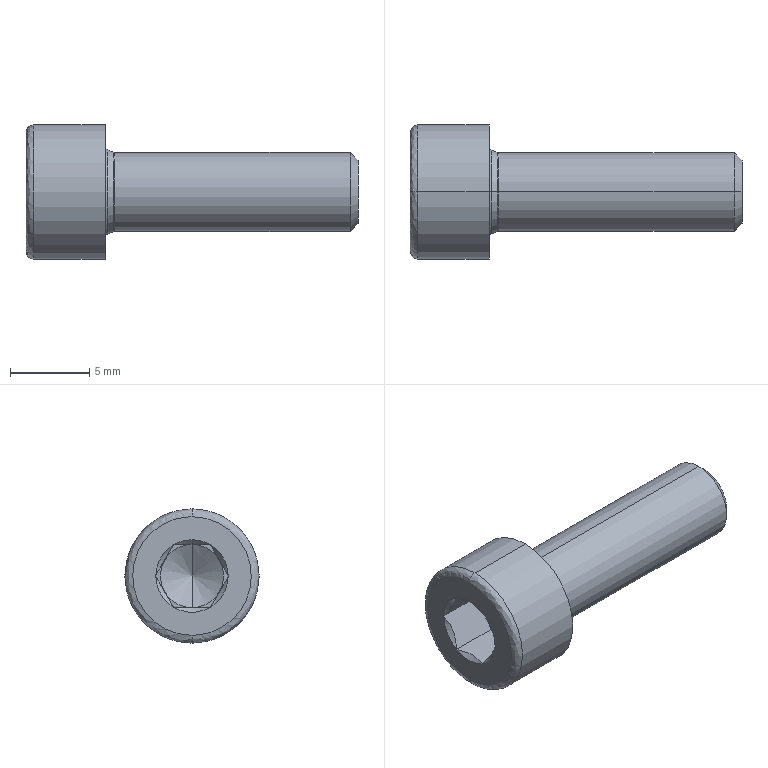Part | STEP file | _Hexagon socket head cap screw DIN 912 - M5x16 | 1 solid | 38 faces | box 21 x 8.5 x 8.5 mm | volume 547.668 mm3 | plane 15 | cone 13 | spline 6 | cylinder 4 | commonest cylinder face diameters 5 x2 8.5 x2
STEP:
#1=CARTESIAN_POINT('',(0.5298,0.,2.513));
#2=VERTEX_POINT('',#1);
#3=CARTESIAN_POINT('',(0.5298,0.,-2.513));
#4=VERTEX_POINT('',#3);
#5=CARTESIAN_POINT('',(0.5298,0.,0.));
#6=DIRECTION('',(-1.,0.,0.));
#7=DIRECTION('',(0.,0.,-1.));
#8=AXIS2_PLACEMENT_3D('',#5,#6,#7);
#9=CIRCLE('',#8,2.513);
#10=EDGE_CURVE('',#2,#4,#9,.T.);
#11=ORIENTED_EDGE('',*,*,#10,.F.);
#12=CARTESIAN_POINT('',(0.6,0.,2.5));
#13=VERTEX_POINT('',#12);
#14=CARTESIAN_POINT('',(0.6,0.,2.7));
#15=DIRECTION('',(0.,-1.,0.));
#16=DIRECTION('',(0.,0.,1.));
#17=AXIS2_PLACEMENT_3D('',#14,#15,#16);
#18=CIRCLE('',#17,0.2);
#19=EDGE_CURVE('',#2,#13,#18,.T.);
#20=ORIENTED_EDGE('',*,*,#19,.T.);
#21=CARTESIAN_POINT('',(0.6,0.,-2.5));
#22=VERTEX_POINT('',#21);
#23=CARTESIAN_POINT('',(0.6,0.,0.));
#24=DIRECTION('',(1.,0.,0.));
#25=DIRECTION('',(0.,0.,1.));
#26=AXIS2_PLACEMENT_3D('',#23,#24,#25);
#27=CIRCLE('',#26,2.5);
#28=EDGE_CURVE('',#22,#13,#27,.T.);
#29=ORIENTED_EDGE('',*,*,#28,.F.);
#30=CARTESIAN_POINT('',(0.6,0.,-2.7));
#31=DIRECTION('',(0.,1.,0.));
#32=DIRECTION('',(0.,0.,-1.));
#33=AXIS2_PLACEMENT_3D('',#30,#31,#32);
#34=CIRCLE('',#33,0.2);
#35=EDGE_CURVE('',#4,#22,#34,.T.);
#36=ORIENTED_EDGE('',*,*,#35,.F.);
#37=EDGE_LOOP('',(#11,#20,#29,#36));
#38=FACE_OUTER_BOUND('',#37,.T.);
#39=CARTESIAN_POINT('',(0.5298,0.,-2.513));
#40=CARTESIAN_POINT('',(0.5298,5.025,-2.513));
#41=CARTESIAN_POINT('',(0.5298,5.025,2.513));
#42=CARTESIAN_POINT('',(0.5298,0.,2.513));
#43=CARTESIAN_POINT('',(0.5523,0.,-2.504));
#44=CARTESIAN_POINT('',(0.5523,5.009,-2.504));
#45=CARTESIAN_POINT('',(0.5523,5.009,2.504));
#46=CARTESIAN_POINT('',(0.5523,0.,2.504));
#47=CARTESIAN_POINT('',(0.576,0.,-2.5));
#48=CARTESIAN_POINT('',(0.576,5.,-2.5));
#49=CARTESIAN_POINT('',(0.576,5.,2.5));
#50=CARTESIAN_POINT('',(0.576,0.,2.5));
#51=CARTESIAN_POINT('',(0.6,0.,-2.5));
#52=CARTESIAN_POINT('',(0.6,5.,-2.5));
#53=CARTESIAN_POINT('',(0.6,5.,2.5));
#54=CARTESIAN_POINT('',(0.6,0.,2.5));
#55=(BOUNDED_SURFACE()B_SPLINE_SURFACE(3,3,((#39,#40,#41,#42),(#43,#44,#45,#46),(#47,#48,#49,#50),(#51,#52,#53,#54)),.UNSPECIFIED.,.F.,.F.,.F.)B_SPLINE_SURFACE_WITH_KNOTS((4,4),(4,4),(0.,1.),(0.,1.),.UNSPECIFIED.)GEOMETRIC_REPRESENTATION_ITEM()RATIONAL_B_SPLINE_SURFACE(((1.,0.3333,0.3333,1.),(0.9893,0.3298,0.3298,0.9893),(0.9893,0.3298,0.3298,0.9893),(1.,0.3333,0.3333,1.)))REPRESENTATION_ITEM('')SURFACE());
#56=ADVANCED_FACE('',(#38),#55,.F.);
#57=CARTESIAN_POINT('',(0.,0.,2.85));
#58=VERTEX_POINT('',#57);
#59=CARTESIAN_POINT('',(0.,0.,-2.85));
#60=VERTEX_POINT('',#59);
#61=CARTESIAN_POINT('',(0.,0.,2.85));
#62=CARTESIAN_POINT('',(0.,0.1814,2.85));
#63=CARTESIAN_POINT('',(0.,0.4486,2.825));
#64=CARTESIAN_POINT('',(0.,0.7517,2.752));
#65=CARTESIAN_POINT('',(0.,0.9011,2.705));
#66=CARTESIAN_POINT('',(0.,0.9647,2.682));
#67=CARTESIAN_POINT('',(0.,1.007,2.666));
#68=CARTESIAN_POINT('',(0.,1.026,2.659));
#69=CARTESIAN_POINT('',(0.,1.415,2.505));
#70=CARTESIAN_POINT('',(0.,1.737,2.294));
#71=CARTESIAN_POINT('',(0.,2.154,1.876));
#72=CARTESIAN_POINT('',(0.,2.338,1.651));
#73=CARTESIAN_POINT('',(0.,2.509,1.359));
#74=CARTESIAN_POINT('',(0.,2.583,1.207));
#75=CARTESIAN_POINT('',(0.,2.612,1.14));
#76=CARTESIAN_POINT('',(0.,2.632,1.095));
#77=CARTESIAN_POINT('',(0.,2.642,1.07));
#78=CARTESIAN_POINT('',(0.,2.783,0.7118));
#79=CARTESIAN_POINT('',(0.,2.85,0.3628));
#80=CARTESIAN_POINT('',(0.,2.85,-0.1814));
#81=CARTESIAN_POINT('',(0.,2.825,-0.4486));
#82=CARTESIAN_POINT('',(0.,2.752,-0.7517));
#83=CARTESIAN_POINT('',(0.,2.705,-0.9011));
#84=CARTESIAN_POINT('',(0.,2.682,-0.9647));
#85=CARTESIAN_POINT('',(0.,2.666,-1.007));
#86=CARTESIAN_POINT('',(0.,2.659,-1.026));
#87=CARTESIAN_POINT('',(0.,2.505,-1.415));
#88=CARTESIAN_POINT('',(0.,2.294,-1.737));
#89=CARTESIAN_POINT('',(0.,1.876,-2.154));
#90=CARTESIAN_POINT('',(0.,1.651,-2.338));
#91=CARTESIAN_POINT('',(0.,1.359,-2.509));
#92=CARTESIAN_POINT('',(0.,1.207,-2.583));
#93=CARTESIAN_POINT('',(0.,1.14,-2.612));
#94=CARTESIAN_POINT('',(0.,1.095,-2.632));
#95=CARTESIAN_POINT('',(0.,1.07,-2.642));
#96=CARTESIAN_POINT('',(0.,0.7119,-2.783));
#97=CARTESIAN_POINT('',(0.,0.3622,-2.85));
#98=CARTESIAN_POINT('',(0.,0.,-2.85));
#99=B_SPLINE_CURVE_WITH_KNOTS('',3,(#61,#62,#63,#64,#65,#66,#67,#68,#69,#70,#71,#72,#73,#74,#75,#76,#77,#78,#79,#80,#81,#82,#83,#84,#85,#86,#87,#88,#89,#90,#91,#92,#93,#94,#95,#96,#97,#98),.UNSPECIFIED.,.F.,.F.,(4,1,1,1,2,2,2,1,1,1,2,2,2,1,1,1,2,2,2,1,1,1,2,2,4),(0.5,0.5312,0.5469,0.5547,0.5586,0.5625,0.625,0.6562,0.6719,0.6797,0.6836,0.6875,0.75,0.7812,0.7969,0.8047,0.8086,0.8125,0.875,0.9062,0.9219,0.9297,0.9336,0.9375,1.),.UNSPECIFIED.);
#100=EDGE_CURVE('',#58,#60,#99,.T.);
#101=ORIENTED_EDGE('',*,*,#100,.F.);
#102=CARTESIAN_POINT('',(0.1298,0.,2.663));
#103=VERTEX_POINT('',#102);
#104=CARTESIAN_POINT('',(0.2,0.,2.85));
#105=DIRECTION('',(0.,-1.,0.));
#106=DIRECTION('',(0.,0.,1.));
#107=AXIS2_PLACEMENT_3D('',#104,#105,#106);
#108=CIRCLE('',#107,0.2);
#109=EDGE_CURVE('',#58,#103,#108,.T.);
#110=ORIENTED_EDGE('',*,*,#109,.T.);
#111=CARTESIAN_POINT('',(0.1298,0.,-2.663));
#112=VERTEX_POINT('',#111);
#113=CARTESIAN_POINT('',(0.1298,0.,0.));
#114=DIRECTION('',(1.,0.,0.));
#115=DIRECTION('',(0.,0.,1.));
#116=AXIS2_PLACEMENT_3D('',#113,#114,#115);
#117=CIRCLE('',#116,2.663);
#118=EDGE_CURVE('',#112,#103,#117,.T.);
#119=ORIENTED_EDGE('',*,*,#118,.F.);
#120=CARTESIAN_POINT('',(0.2,0.,-2.85));
#121=DIRECTION('',(0.,1.,0.));
#122=DIRECTION('',(0.,0.,-1.));
#123=AXIS2_PLACEMENT_3D('',#120,#121,#122);
#124=CIRCLE('',#123,0.2);
#125=EDGE_CURVE('',#60,#112,#124,.T.);
#126=ORIENTED_EDGE('',*,*,#125,.F.);
#127=EDGE_LOOP('',(#101,#110,#119,#126));
#128=FACE_OUTER_BOUND('',#127,.T.);
#129=CARTESIAN_POINT('',(0.,0.,-2.85));
#130=CARTESIAN_POINT('',(0.,5.7,-2.85));
#131=CARTESIAN_POINT('',(0.,5.7,2.85));
#132=CARTESIAN_POINT('',(0.,0.,2.85));
#133=CARTESIAN_POINT('',(0.,0.,-2.764));
#134=CARTESIAN_POINT('',(0.,5.528,-2.764));
#135=CARTESIAN_POINT('',(0.,5.528,2.764));
#136=CARTESIAN_POINT('',(0.,0.,2.764));
#137=CARTESIAN_POINT('',(0.04909,0.,-2.693));
#138=CARTESIAN_POINT('',(0.04909,5.386,-2.693));
#139=CARTESIAN_POINT('',(0.04909,5.386,2.693));
#140=CARTESIAN_POINT('',(0.04909,0.,2.693));
#141=CARTESIAN_POINT('',(0.1298,0.,-2.663));
#142=CARTESIAN_POINT('',(0.1298,5.325,-2.663));
#143=CARTESIAN_POINT('',(0.1298,5.325,2.663));
#144=CARTESIAN_POINT('',(0.1298,0.,2.663));
#145=(BOUNDED_SURFACE()B_SPLINE_SURFACE(3,3,((#129,#130,#131,#132),(#133,#134,#135,#136),(#137,#138,#139,#140),(#141,#142,#143,#144)),.UNSPECIFIED.,.F.,.F.,.T.)B_SPLINE_SURFACE_WITH_KNOTS((4,4),(4,4),(0.,1.),(0.,1.),.UNSPECIFIED.)GEOMETRIC_REPRESENTATION_ITEM()RATIONAL_B_SPLINE_SURFACE(((1.,0.3333,0.3333,1.),(0.8813,0.2938,0.2938,0.8813),(0.8813,0.2938,0.2938,0.8813),(1.,0.3333,0.3333,1.)))REPRESENTATION_ITEM('')SURFACE());
#146=ADVANCED_FACE('',(#128),#145,.F.);
#147=CARTESIAN_POINT('',(-4.5,0.,4.25));
#148=VERTEX_POINT('',#147);
#149=CARTESIAN_POINT('',(-4.5,0.,-4.25));
#150=VERTEX_POINT('',#149);
#151=CARTESIAN_POINT('',(-4.5,0.,0.));
#152=DIRECTION('',(1.,0.,0.));
#153=DIRECTION('',(0.,0.,1.));
#154=AXIS2_PLACEMENT_3D('',#151,#152,#153);
#155=CIRCLE('',#154,4.25);
#156=EDGE_CURVE('',#148,#150,#155,.T.);
#157=ORIENTED_EDGE('',*,*,#156,.F.);
#158=CARTESIAN_POINT('',(-5.,0.,3.75));
#159=VERTEX_POINT('',#158);
#160=CARTESIAN_POINT('',(-4.5,0.,3.75));
#161=DIRECTION('',(0.,-1.,0.));
#162=DIRECTION('',(0.,0.,1.));
#163=AXIS2_PLACEMENT_3D('',#160,#161,#162);
#164=CIRCLE('',#163,0.5);
#165=EDGE_CURVE('',#148,#159,#164,.T.);
#166=ORIENTED_EDGE('',*,*,#165,.T.);
#167=CARTESIAN_POINT('',(-5.,0.,-3.75));
#168=VERTEX_POINT('',#167);
#169=CARTESIAN_POINT('',(-5.,0.,3.75));
#170=CARTESIAN_POINT('',(-5.,-7.5,3.75));
#171=CARTESIAN_POINT('',(-5.,-7.5,-3.75));
#172=CARTESIAN_POINT('',(-5.,0.,-3.75));
#173=(BOUNDED_CURVE()B_SPLINE_CURVE(3,(#169,#170,#171,#172),.UNSPECIFIED.,.F.,.F.)B_SPLINE_CURVE_WITH_KNOTS((4,4),(0.5,1.),.UNSPECIFIED.)CURVE()GEOMETRIC_REPRESENTATION_ITEM()RATIONAL_B_SPLINE_CURVE((1.,0.3333,0.3333,1.))REPRESENTATION_ITEM(''));
#174=EDGE_CURVE('',#159,#168,#173,.T.);
#175=ORIENTED_EDGE('',*,*,#174,.T.);
#176=CARTESIAN_POINT('',(-4.5,0.,-3.75));
#177=DIRECTION('',(0.,1.,0.));
#178=DIRECTION('',(0.,0.,-1.));
#179=AXIS2_PLACEMENT_3D('',#176,#177,#178);
#180=CIRCLE('',#179,0.5);
#181=EDGE_CURVE('',#150,#168,#180,.T.);
#182=ORIENTED_EDGE('',*,*,#181,.F.);
#183=EDGE_LOOP('',(#157,#166,#175,#182));
#184=FACE_OUTER_BOUND('',#183,.T.);
#185=CARTESIAN_POINT('',(-4.5,0.,4.25));
#186=CARTESIAN_POINT('',(-4.5,-8.5,4.25));
#187=CARTESIAN_POINT('',(-4.5,-8.5,-4.25));
#188=CARTESIAN_POINT('',(-4.5,0.,-4.25));
#189=CARTESIAN_POINT('',(-4.793,0.,4.25));
#190=CARTESIAN_POINT('',(-4.793,-8.5,4.25));
#191=CARTESIAN_POINT('',(-4.793,-8.5,-4.25));
#192=CARTESIAN_POINT('',(-4.793,0.,-4.25));
#193=CARTESIAN_POINT('',(-5.,0.,4.043));
#194=CARTESIAN_POINT('',(-5.,-8.086,4.043));
#195=CARTESIAN_POINT('',(-5.,-8.086,-4.043));
#196=CARTESIAN_POINT('',(-5.,0.,-4.043));
#197=CARTESIAN_POINT('',(-5.,0.,3.75));
#198=CARTESIAN_POINT('',(-5.,-7.5,3.75));
#199=CARTESIAN_POINT('',(-5.,-7.5,-3.75));
#200=CARTESIAN_POINT('',(-5.,0.,-3.75));
#201=(BOUNDED_SURFACE()B_SPLINE_SURFACE(3,3,((#185,#186,#187,#188),(#189,#190,#191,#192),(#193,#194,#195,#196),(#197,#198,#199,#200)),.UNSPECIFIED.,.F.,.F.,.F.)B_SPLINE_SURFACE_WITH_KNOTS((4,4),(4,4),(0.,1.),(0.,1.),.UNSPECIFIED.)GEOMETRIC_REPRESENTATION_ITEM()RATIONAL_B_SPLINE_SURFACE(((1.,0.3333,0.3333,1.),(0.8047,0.2682,0.2682,0.8047),(0.8047,0.2682,0.2682,0.8047),(1.,0.3333,0.3333,1.)))REPRESENTATION_ITEM('')SURFACE());
#202=ADVANCED_FACE('',(#184),#201,.T.);
#203=CARTESIAN_POINT('',(15.509,0.,2.5));
#204=VERTEX_POINT('',#203);
#205=CARTESIAN_POINT('',(15.509,0.,-2.5));
#206=VERTEX_POINT('',#205);
#207=CARTESIAN_POINT('',(15.509,0.,0.));
#208=DIRECTION('',(-1.,0.,0.));
#209=DIRECTION('',(0.,0.,1.));
#210=AXIS2_PLACEMENT_3D('',#207,#208,#209);
#211=CIRCLE('',#210,2.5);
#212=EDGE_CURVE('',#204,#206,#211,.T.);
#213=ORIENTED_EDGE('',*,*,#212,.T.);
#214=CARTESIAN_POINT('',(19.,0.,-2.5));
#215=DIRECTION('',(-1.,0.,0.));
#216=VECTOR('',#215,1000.);
#217=LINE('',#214,#216);
#218=EDGE_CURVE('',#206,#22,#217,.T.);
#219=ORIENTED_EDGE('',*,*,#218,.T.);
#220=ORIENTED_EDGE('',*,*,#28,.T.);
#221=CARTESIAN_POINT('',(19.,0.,2.5));
#222=DIRECTION('',(-1.,0.,0.));
#223=VECTOR('',#222,1000.);
#224=LINE('',#221,#223);
#225=EDGE_CURVE('',#204,#13,#224,.T.);
#226=ORIENTED_EDGE('',*,*,#225,.F.);
#227=EDGE_LOOP('',(#213,#219,#220,#226));
#228=FACE_OUTER_BOUND('',#227,.T.);
#229=CARTESIAN_POINT('',(19.,0.,0.));
#230=DIRECTION('',(-1.,0.,0.));
#231=DIRECTION('',(0.,0.,1.));
#232=AXIS2_PLACEMENT_3D('',#229,#230,#231);
#233=CYLINDRICAL_SURFACE('',#232,2.5);
#234=ADVANCED_FACE('',(#228),#233,.T.);
#235=CARTESIAN_POINT('',(16.,0.,2.009));
#236=VERTEX_POINT('',#235);
#237=CARTESIAN_POINT('',(16.,0.,-2.009));
#238=VERTEX_POINT('',#237);
#239=CARTESIAN_POINT('',(16.,0.,0.));
#240=DIRECTION('',(-1.,0.,0.));
#241=DIRECTION('',(0.,0.,1.));
#242=AXIS2_PLACEMENT_3D('',#239,#240,#241);
#243=CIRCLE('',#242,2.009);
#244=EDGE_CURVE('',#236,#238,#243,.T.);
#245=ORIENTED_EDGE('',*,*,#244,.T.);
#246=CARTESIAN_POINT('',(15.51,0.,-2.5));
#247=DIRECTION('',(-0.7071,0.,-0.7071));
#248=VECTOR('',#247,1000.);
#249=LINE('',#246,#248);
#250=EDGE_CURVE('',#238,#206,#249,.T.);
#251=ORIENTED_EDGE('',*,*,#250,.T.);
#252=ORIENTED_EDGE('',*,*,#212,.F.);
#253=CARTESIAN_POINT('',(15.51,0.,2.5));
#254=DIRECTION('',(-0.7071,0.,0.7071));
#255=VECTOR('',#254,1000.);
#256=LINE('',#253,#255);
#257=EDGE_CURVE('',#236,#204,#256,.T.);
#258=ORIENTED_EDGE('',*,*,#257,.F.);
#259=EDGE_LOOP('',(#245,#251,#252,#258));
#260=FACE_OUTER_BOUND('',#259,.T.);
#261=CARTESIAN_POINT('',(15.51,0.,0.));
#262=DIRECTION('',(-1.,0.,0.));
#263=DIRECTION('',(0.,0.,1.));
#264=AXIS2_PLACEMENT_3D('',#261,#262,#263);
#265=CONICAL_SURFACE('',#264,2.5,0.7854);
#266=ADVANCED_FACE('',(#260),#265,.T.);
#267=ORIENTED_EDGE('',*,*,#10,.T.);
#268=CARTESIAN_POINT('',(0.1298,0.,-2.663));
#269=DIRECTION('',(-0.9363,0.,-0.3511));
#270=VECTOR('',#269,1000.);
#271=LINE('',#268,#270);
#272=EDGE_CURVE('',#4,#112,#271,.T.);
#273=ORIENTED_EDGE('',*,*,#272,.T.);
#274=ORIENTED_EDGE('',*,*,#118,.T.);
#275=CARTESIAN_POINT('',(0.1298,0.,2.663));
#276=DIRECTION('',(-0.9363,0.,0.3511));
#277=VECTOR('',#276,1000.);
#278=LINE('',#275,#277);
#279=EDGE_CURVE('',#2,#103,#278,.T.);
#280=ORIENTED_EDGE('',*,*,#279,.F.);
#281=EDGE_LOOP('',(#267,#273,#274,#280));
#282=FACE_OUTER_BOUND('',#281,.T.);
#283=CARTESIAN_POINT('',(0.1298,0.,0.));
#284=DIRECTION('',(-1.,0.,0.));
#285=DIRECTION('',(0.,0.,1.));
#286=AXIS2_PLACEMENT_3D('',#283,#284,#285);
#287=CONICAL_SURFACE('',#286,2.663,0.3588);
#288=ADVANCED_FACE('',(#282),#287,.T.);
#289=CARTESIAN_POINT('',(0.,0.,4.25));
#290=VERTEX_POINT('',#289);
#291=CARTESIAN_POINT('',(0.,0.,-4.25));
#292=VERTEX_POINT('',#291);
#293=CARTESIAN_POINT('',(0.,0.,0.));
#294=DIRECTION('',(-1.,0.,0.));
#295=DIRECTION('',(0.,0.,1.));
#296=AXIS2_PLACEMENT_3D('',#293,#294,#295);
#297=CIRCLE('',#296,4.25);
#298=EDGE_CURVE('',#290,#292,#297,.T.);
#299=ORIENTED_EDGE('',*,*,#298,.T.);
#300=CARTESIAN_POINT('',(19.,0.,-4.25));
#301=DIRECTION('',(-1.,0.,0.));
#302=VECTOR('',#301,1000.);
#303=LINE('',#300,#302);
#304=EDGE_CURVE('',#292,#150,#303,.T.);
#305=ORIENTED_EDGE('',*,*,#304,.T.);
#306=CARTESIAN_POINT('',(-4.5,0.,0.));
#307=DIRECTION('',(1.,0.,0.));
#308=DIRECTION('',(0.,0.,1.));
#309=AXIS2_PLACEMENT_3D('',#306,#307,#308);
#310=CIRCLE('',#309,4.25);
#311=EDGE_CURVE('',#150,#148,#310,.T.);
#312=ORIENTED_EDGE('',*,*,#311,.T.);
#313=CARTESIAN_POINT('',(19.,0.,4.25));
#314=DIRECTION('',(-1.,0.,0.));
#315=VECTOR('',#314,1000.);
#316=LINE('',#313,#315);
#317=EDGE_CURVE('',#290,#148,#316,.T.);
#318=ORIENTED_EDGE('',*,*,#317,.F.);
#319=EDGE_LOOP('',(#299,#305,#312,#318));
#320=FACE_OUTER_BOUND('',#319,.T.);
#321=CARTESIAN_POINT('',(19.,0.,0.));
#322=DIRECTION('',(-1.,0.,0.));
#323=DIRECTION('',(0.,0.,1.));
#324=AXIS2_PLACEMENT_3D('',#321,#322,#323);
#325=CYLINDRICAL_SURFACE('',#324,4.25);
#326=ADVANCED_FACE('',(#320),#325,.T.);
#327=CARTESIAN_POINT('',(-4.71,0.,2.));
#328=VERTEX_POINT('',#327);
#329=CARTESIAN_POINT('',(-5.,1.115,2.));
#330=VERTEX_POINT('',#329);
#331=CARTESIAN_POINT('',(-4.71,0.,2.));
#332=CARTESIAN_POINT('',(-4.71,0.3872,2.));
#333=CARTESIAN_POINT('',(-4.829,0.765,2.));
#334=CARTESIAN_POINT('',(-5.,1.115,2.));
#335=B_SPLINE_CURVE_WITH_KNOTS('',3,(#331,#332,#333,#334),.UNSPECIFIED.,.F.,.F.,(4,4),(0.001154,0.0023),.UNSPECIFIED.);
#336=EDGE_CURVE('',#328,#330,#335,.T.);
#337=ORIENTED_EDGE('',*,*,#336,.F.);
#338=CARTESIAN_POINT('',(-5.,0.,2.29));
#339=VERTEX_POINT('',#338);
#340=CARTESIAN_POINT('',(-5.,0.,2.29));
#341=DIRECTION('',(-0.7071,0.,0.7071));
#342=VECTOR('',#341,1000.);
#343=LINE('',#340,#342);
#344=EDGE_CURVE('',#328,#339,#343,.T.);
#345=ORIENTED_EDGE('',*,*,#344,.T.);
#346=CARTESIAN_POINT('',(-5.,0.,0.));
#347=DIRECTION('',(-1.,0.,0.));
#348=DIRECTION('',(0.,0.,1.));
#349=AXIS2_PLACEMENT_3D('',#346,#347,#348);
#350=CIRCLE('',#349,2.29);
#351=EDGE_CURVE('',#339,#330,#350,.T.);
#352=ORIENTED_EDGE('',*,*,#351,.T.);
#353=EDGE_LOOP('',(#337,#345,#352));
#354=FACE_OUTER_BOUND('',#353,.T.);
#355=CARTESIAN_POINT('',(-5.,0.,0.));
#356=DIRECTION('',(-1.,0.,0.));
#357=DIRECTION('',(0.,0.,1.));
#358=AXIS2_PLACEMENT_3D('',#355,#356,#357);
#359=CONICAL_SURFACE('',#358,2.29,0.7854);
#360=ADVANCED_FACE('',(#354),#359,.F.);
#361=CARTESIAN_POINT('',(-0.7453,0.,0.));
#362=VERTEX_POINT('',#361);
#363=CARTESIAN_POINT('',(-1.9,0.,2.));
#364=VERTEX_POINT('',#363);
#365=CARTESIAN_POINT('',(-1.9,0.,2.));
#366=DIRECTION('',(-0.5,0.,0.866));
#367=VECTOR('',#366,1000.);
#368=LINE('',#365,#367);
#369=EDGE_CURVE('',#362,#364,#368,.T.);
#370=ORIENTED_EDGE('',*,*,#369,.F.);
#371=CARTESIAN_POINT('',(-1.9,0.,-2.));
#372=VERTEX_POINT('',#371);
#373=CARTESIAN_POINT('',(-1.9,0.,-2.));
#374=DIRECTION('',(-0.5,0.,-0.866));
#375=VECTOR('',#374,1000.);
#376=LINE('',#373,#375);
#377=EDGE_CURVE('',#362,#372,#376,.T.);
#378=ORIENTED_EDGE('',*,*,#377,.T.);
#379=CARTESIAN_POINT('',(-1.9,-1.732,-1.));
#380=VERTEX_POINT('',#379);
#381=CARTESIAN_POINT('',(-1.9,0.,0.));
#382=DIRECTION('',(1.,0.,0.));
#383=DIRECTION('',(0.,0.,1.));
#384=AXIS2_PLACEMENT_3D('',#381,#382,#383);
#385=CIRCLE('',#384,2.);
#386=EDGE_CURVE('',#380,#372,#385,.T.);
#387=ORIENTED_EDGE('',*,*,#386,.F.);
#388=CARTESIAN_POINT('',(-1.9,-1.732,1.));
#389=VERTEX_POINT('',#388);
#390=CARTESIAN_POINT('',(-1.9,0.,0.));
#391=DIRECTION('',(1.,0.,0.));
#392=DIRECTION('',(0.,0.,1.));
#393=AXIS2_PLACEMENT_3D('',#390,#391,#392);
#394=CIRCLE('',#393,2.);
#395=EDGE_CURVE('',#389,#380,#394,.T.);
#396=ORIENTED_EDGE('',*,*,#395,.F.);
#397=CARTESIAN_POINT('',(-1.9,0.,0.));
#398=DIRECTION('',(1.,0.,0.));
#399=DIRECTION('',(0.,0.,1.));
#400=AXIS2_PLACEMENT_3D('',#397,#398,#399);
#401=CIRCLE('',#400,2.);
#402=EDGE_CURVE('',#364,#389,#401,.T.);
#403=ORIENTED_EDGE('',*,*,#402,.F.);
#404=EDGE_LOOP('',(#370,#378,#387,#396,#403));
#405=FACE_OUTER_BOUND('',#404,.T.);
#406=CARTESIAN_POINT('',(-1.9,0.,0.));
#407=DIRECTION('',(-1.,0.,0.));
#408=DIRECTION('',(0.,0.,1.));
#409=AXIS2_PLACEMENT_3D('',#406,#407,#408);
#410=CONICAL_SURFACE('',#409,2.,1.047);
#411=ADVANCED_FACE('',(#405),#410,.F.);
#412=ORIENTED_EDGE('',*,*,#218,.F.);
#413=CARTESIAN_POINT('',(15.509,0.,0.));
#414=DIRECTION('',(-1.,0.,0.));
#415=DIRECTION('',(0.,0.,1.));
#416=AXIS2_PLACEMENT_3D('',#413,#414,#415);
#417=CIRCLE('',#416,2.5);
#418=EDGE_CURVE('',#206,#204,#417,.T.);
#419=ORIENTED_EDGE('',*,*,#418,.T.);
#420=ORIENTED_EDGE('',*,*,#225,.T.);
#421=CARTESIAN_POINT('',(0.6,0.,0.));
#422=DIRECTION('',(1.,0.,0.));
#423=DIRECTION('',(0.,0.,1.));
#424=AXIS2_PLACEMENT_3D('',#421,#422,#423);
#425=CIRCLE('',#424,2.5);
#426=EDGE_CURVE('',#13,#22,#425,.T.);
#427=ORIENTED_EDGE('',*,*,#426,.T.);
#428=EDGE_LOOP('',(#412,#419,#420,#427));
#429=FACE_OUTER_BOUND('',#428,.T.);
#430=CARTESIAN_POINT('',(19.,0.,0.));
#431=DIRECTION('',(-1.,0.,0.));
#432=DIRECTION('',(0.,0.,1.));
#433=AXIS2_PLACEMENT_3D('',#430,#431,#432);
#434=CYLINDRICAL_SURFACE('',#433,2.5);
#435=ADVANCED_FACE('',(#429),#434,.T.);
#436=ORIENTED_EDGE('',*,*,#19,.F.);
#437=CARTESIAN_POINT('',(0.5298,0.,0.));
#438=DIRECTION('',(-1.,0.,0.));
#439=DIRECTION('',(0.,0.,-1.));
#440=AXIS2_PLACEMENT_3D('',#437,#438,#439);
#441=CIRCLE('',#440,2.513);
#442=EDGE_CURVE('',#4,#2,#441,.T.);
#443=ORIENTED_EDGE('',*,*,#442,.F.);
#444=ORIENTED_EDGE('',*,*,#35,.T.);
#445=ORIENTED_EDGE('',*,*,#426,.F.);
#446=EDGE_LOOP('',(#436,#443,#444,#445));
#447=FACE_OUTER_BOUND('',#446,.T.);
#448=CARTESIAN_POINT('',(0.5298,0.,2.513));
#449=CARTESIAN_POINT('',(0.5298,-5.025,2.513));
#450=CARTESIAN_POINT('',(0.5298,-5.025,-2.513));
#451=CARTESIAN_POINT('',(0.5298,0.,-2.513));
#452=CARTESIAN_POINT('',(0.5523,0.,2.504));
#453=CARTESIAN_POINT('',(0.5523,-5.009,2.504));
#454=CARTESIAN_POINT('',(0.5523,-5.009,-2.504));
#455=CARTESIAN_POINT('',(0.5523,0.,-2.504));
#456=CARTESIAN_POINT('',(0.576,0.,2.5));
#457=CARTESIAN_POINT('',(0.576,-5.,2.5));
#458=CARTESIAN_POINT('',(0.576,-5.,-2.5));
#459=CARTESIAN_POINT('',(0.576,0.,-2.5));
#460=CARTESIAN_POINT('',(0.6,0.,2.5));
#461=CARTESIAN_POINT('',(0.6,-5.,2.5));
#462=CARTESIAN_POINT('',(0.6,-5.,-2.5));
#463=CARTESIAN_POINT('',(0.6,0.,-2.5));
#464=(BOUNDED_SURFACE()B_SPLINE_SURFACE(3,3,((#448,#449,#450,#451),(#452,#453,#454,#455),(#456,#457,#458,#459),(#460,#461,#462,#463)),.UNSPECIFIED.,.F.,.F.,.F.)B_SPLINE_SURFACE_WITH_KNOTS((4,4),(4,4),(0.,1.),(0.,1.),.UNSPECIFIED.)GEOMETRIC_REPRESENTATION_ITEM()RATIONAL_B_SPLINE_SURFACE(((1.,0.3333,0.3333,1.),(0.9893,0.3298,0.3298,0.9893),(0.9893,0.3298,0.3298,0.9893),(1.,0.3333,0.3333,1.)))REPRESENTATION_ITEM('')SURFACE());
#465=ADVANCED_FACE('',(#447),#464,.F.);
#466=ORIENTED_EDGE('',*,*,#250,.F.);
#467=CARTESIAN_POINT('',(16.,0.,0.));
#468=DIRECTION('',(-1.,0.,0.));
#469=DIRECTION('',(0.,0.,1.));
#470=AXIS2_PLACEMENT_3D('',#467,#468,#469);
#471=CIRCLE('',#470,2.009);
#472=EDGE_CURVE('',#238,#236,#471,.T.);
#473=ORIENTED_EDGE('',*,*,#472,.T.);
#474=ORIENTED_EDGE('',*,*,#257,.T.);
#475=ORIENTED_EDGE('',*,*,#418,.F.);
#476=EDGE_LOOP('',(#466,#473,#474,#475));
#477=FACE_OUTER_BOUND('',#476,.T.);
#478=CARTESIAN_POINT('',(15.51,0.,0.));
#479=DIRECTION('',(-1.,0.,0.));
#480=DIRECTION('',(0.,0.,1.));
#481=AXIS2_PLACEMENT_3D('',#478,#479,#480);
#482=CONICAL_SURFACE('',#481,2.5,0.7854);
#483=ADVANCED_FACE('',(#477),#482,.T.);
#484=ORIENTED_EDGE('',*,*,#272,.F.);
#485=ORIENTED_EDGE('',*,*,#442,.T.);
#486=ORIENTED_EDGE('',*,*,#279,.T.);
#487=CARTESIAN_POINT('',(0.1298,0.,0.));
#488=DIRECTION('',(1.,0.,0.));
#489=DIRECTION('',(0.,0.,1.));
#490=AXIS2_PLACEMENT_3D('',#487,#488,#489);
#491=CIRCLE('',#490,2.663);
#492=EDGE_CURVE('',#103,#112,#491,.T.);
#493=ORIENTED_EDGE('',*,*,#492,.T.);
#494=EDGE_LOOP('',(#484,#485,#486,#493));
#495=FACE_OUTER_BOUND('',#494,.T.);
#496=CARTESIAN_POINT('',(0.1298,0.,0.));
#497=DIRECTION('',(-1.,0.,0.));
#498=DIRECTION('',(0.,0.,1.));
#499=AXIS2_PLACEMENT_3D('',#496,#497,#498);
#500=CONICAL_SURFACE('',#499,2.663,0.3588);
#501=ADVANCED_FACE('',(#495),#500,.T.);
#502=ORIENTED_EDGE('',*,*,#244,.F.);
#503=ORIENTED_EDGE('',*,*,#472,.F.);
#504=EDGE_LOOP('',(#502,#503));
#505=FACE_OUTER_BOUND('',#504,.T.);
#506=CARTESIAN_POINT('',(16.,2.01,0.));
#507=DIRECTION('',(-1.,0.,0.));
#508=DIRECTION('',(0.,0.,1.));
#509=AXIS2_PLACEMENT_3D('',#506,#507,#508);
#510=PLANE('',#509);
#511=ADVANCED_FACE('',(#505),#510,.F.);
#512=ORIENTED_EDGE('',*,*,#109,.F.);
#513=CARTESIAN_POINT('',(0.,0.,-2.85));
#514=CARTESIAN_POINT('',(0.,-0.1813,-2.85));
#515=CARTESIAN_POINT('',(0.,-0.4484,-2.825));
#516=CARTESIAN_POINT('',(0.,-0.7516,-2.752));
#517=CARTESIAN_POINT('',(0.,-0.901,-2.705));
#518=CARTESIAN_POINT('',(0.,-0.9646,-2.682));
#519=CARTESIAN_POINT('',(0.,-1.007,-2.666));
#520=CARTESIAN_POINT('',(0.,-1.026,-2.659));
#521=CARTESIAN_POINT('',(0.,-1.415,-2.505));
#522=CARTESIAN_POINT('',(0.,-1.737,-2.294));
#523=CARTESIAN_POINT('',(0.,-2.154,-1.876));
#524=CARTESIAN_POINT('',(0.,-2.338,-1.651));
#525=CARTESIAN_POINT('',(0.,-2.509,-1.359));
#526=CARTESIAN_POINT('',(0.,-2.583,-1.207));
#527=CARTESIAN_POINT('',(0.,-2.612,-1.14));
#528=CARTESIAN_POINT('',(0.,-2.632,-1.095));
#529=CARTESIAN_POINT('',(0.,-2.642,-1.07));
#530=CARTESIAN_POINT('',(0.,-2.783,-0.7118));
#531=CARTESIAN_POINT('',(0.,-2.85,-0.3628));
#532=CARTESIAN_POINT('',(0.,-2.85,0.1814));
#533=CARTESIAN_POINT('',(0.,-2.825,0.4486));
#534=CARTESIAN_POINT('',(0.,-2.752,0.7517));
#535=CARTESIAN_POINT('',(0.,-2.705,0.9011));
#536=CARTESIAN_POINT('',(0.,-2.682,0.9647));
#537=CARTESIAN_POINT('',(0.,-2.666,1.007));
#538=CARTESIAN_POINT('',(0.,-2.659,1.026));
#539=CARTESIAN_POINT('',(0.,-2.505,1.415));
#540=CARTESIAN_POINT('',(0.,-2.294,1.737));
#541=CARTESIAN_POINT('',(0.,-1.876,2.154));
#542=CARTESIAN_POINT('',(0.,-1.651,2.338));
#543=CARTESIAN_POINT('',(0.,-1.359,2.509));
#544=CARTESIAN_POINT('',(0.,-1.207,2.583));
#545=CARTESIAN_POINT('',(0.,-1.14,2.612));
#546=CARTESIAN_POINT('',(0.,-1.095,2.632));
#547=CARTESIAN_POINT('',(0.,-1.07,2.642));
#548=CARTESIAN_POINT('',(0.,-0.7118,2.783));
#549=CARTESIAN_POINT('',(0.,-0.3628,2.85));
#550=CARTESIAN_POINT('',(0.,0.,2.85));
#551=B_SPLINE_CURVE_WITH_KNOTS('',3,(#513,#514,#515,#516,#517,#518,#519,#520,#521,#522,#523,#524,#525,#526,#527,#528,#529,#530,#531,#532,#533,#534,#535,#536,#537,#538,#539,#540,#541,#542,#543,#544,#545,#546,#547,#548,#549,#550),.UNSPECIFIED.,.F.,.F.,(4,1,1,1,2,2,2,1,1,1,2,2,2,1,1,1,2,2,2,1,1,1,2,2,4),(0.,0.03125,0.04687,0.05469,0.05859,0.0625,0.125,0.1563,0.1719,0.1797,0.1836,0.1875,0.25,0.2813,0.2969,0.3047,0.3086,0.3125,0.375,0.4063,0.4219,0.4297,0.4336,0.4375,0.5),.UNSPECIFIED.);
#552=EDGE_CURVE('',#60,#58,#551,.T.);
#553=ORIENTED_EDGE('',*,*,#552,.F.);
#554=ORIENTED_EDGE('',*,*,#125,.T.);
#555=ORIENTED_EDGE('',*,*,#492,.F.);
#556=EDGE_LOOP('',(#512,#553,#554,#555));
#557=FACE_OUTER_BOUND('',#556,.T.);
#558=CARTESIAN_POINT('',(0.,0.,2.85));
#559=CARTESIAN_POINT('',(0.,-5.7,2.85));
#560=CARTESIAN_POINT('',(0.,-5.7,-2.85));
#561=CARTESIAN_POINT('',(0.,0.,-2.85));
#562=CARTESIAN_POINT('',(0.,0.,2.764));
#563=CARTESIAN_POINT('',(0.,-5.528,2.764));
#564=CARTESIAN_POINT('',(0.,-5.528,-2.764));
#565=CARTESIAN_POINT('',(0.,0.,-2.764));
#566=CARTESIAN_POINT('',(0.04909,0.,2.693));
#567=CARTESIAN_POINT('',(0.04909,-5.386,2.693));
#568=CARTESIAN_POINT('',(0.04909,-5.386,-2.693));
#569=CARTESIAN_POINT('',(0.04909,0.,-2.693));
#570=CARTESIAN_POINT('',(0.1298,0.,2.663));
#571=CARTESIAN_POINT('',(0.1298,-5.325,2.663));
#572=CARTESIAN_POINT('',(0.1298,-5.325,-2.663));
#573=CARTESIAN_POINT('',(0.1298,0.,-2.663));
#574=(BOUNDED_SURFACE()B_SPLINE_SURFACE(3,3,((#558,#559,#560,#561),(#562,#563,#564,#565),(#566,#567,#568,#569),(#570,#571,#572,#573)),.UNSPECIFIED.,.F.,.F.,.F.)B_SPLINE_SURFACE_WITH_KNOTS((4,4),(4,4),(0.,1.),(0.,1.),.UNSPECIFIED.)GEOMETRIC_REPRESENTATION_ITEM()RATIONAL_B_SPLINE_SURFACE(((1.,0.3333,0.3333,1.),(0.8813,0.2938,0.2938,0.8813),(0.8813,0.2938,0.2938,0.8813),(1.,0.3333,0.3333,1.)))REPRESENTATION_ITEM('')SURFACE());
#575=ADVANCED_FACE('',(#557),#574,.F.);
#576=ORIENTED_EDGE('',*,*,#298,.F.);
#577=CARTESIAN_POINT('',(0.,0.,0.));
#578=DIRECTION('',(-1.,0.,0.));
#579=DIRECTION('',(0.,0.,1.));
#580=AXIS2_PLACEMENT_3D('',#577,#578,#579);
#581=CIRCLE('',#580,4.25);
#582=EDGE_CURVE('',#292,#290,#581,.T.);
#583=ORIENTED_EDGE('',*,*,#582,.F.);
#584=EDGE_LOOP('',(#576,#583));
#585=FACE_OUTER_BOUND('',#584,.T.);
#586=ORIENTED_EDGE('',*,*,#552,.T.);
#587=ORIENTED_EDGE('',*,*,#100,.T.);
#588=EDGE_LOOP('',(#586,#587));
#589=FACE_BOUND('',#588,.T.);
#590=CARTESIAN_POINT('',(0.,4.25,0.));
#591=DIRECTION('',(-1.,0.,0.));
#592=DIRECTION('',(0.,0.,1.));
#593=AXIS2_PLACEMENT_3D('',#590,#591,#592);
#594=PLANE('',#593);
#595=ADVANCED_FACE('',(#585,#589),#594,.F.);
#596=ORIENTED_EDGE('',*,*,#304,.F.);
#597=ORIENTED_EDGE('',*,*,#582,.T.);
#598=ORIENTED_EDGE('',*,*,#317,.T.);
#599=ORIENTED_EDGE('',*,*,#156,.T.);
#600=EDGE_LOOP('',(#596,#597,#598,#599));
#601=FACE_OUTER_BOUND('',#600,.T.);
#602=CARTESIAN_POINT('',(19.,0.,0.));
#603=DIRECTION('',(-1.,0.,0.));
#604=DIRECTION('',(0.,0.,1.));
#605=AXIS2_PLACEMENT_3D('',#602,#603,#604);
#606=CYLINDRICAL_SURFACE('',#605,4.25);
#607=ADVANCED_FACE('',(#601),#606,.T.);
#608=ORIENTED_EDGE('',*,*,#165,.F.);
#609=ORIENTED_EDGE('',*,*,#311,.F.);
#610=ORIENTED_EDGE('',*,*,#181,.T.);
#611=CARTESIAN_POINT('',(-5.,0.,-3.75));
#612=CARTESIAN_POINT('',(-5.,7.5,-3.75));
#613=CARTESIAN_POINT('',(-5.,7.5,3.75));
#614=CARTESIAN_POINT('',(-5.,0.,3.75));
#615=(BOUNDED_CURVE()B_SPLINE_CURVE(3,(#611,#612,#613,#614),.UNSPECIFIED.,.F.,.T.)B_SPLINE_CURVE_WITH_KNOTS((4,4),(0.,0.5),.UNSPECIFIED.)CURVE()GEOMETRIC_REPRESENTATION_ITEM()RATIONAL_B_SPLINE_CURVE((1.,0.3333,0.3333,1.))REPRESENTATION_ITEM(''));
#616=EDGE_CURVE('',#168,#159,#615,.T.);
#617=ORIENTED_EDGE('',*,*,#616,.T.);
#618=EDGE_LOOP('',(#608,#609,#610,#617));
#619=FACE_OUTER_BOUND('',#618,.T.);
#620=CARTESIAN_POINT('',(-4.5,0.,-4.25));
#621=CARTESIAN_POINT('',(-4.5,8.5,-4.25));
#622=CARTESIAN_POINT('',(-4.5,8.5,4.25));
#623=CARTESIAN_POINT('',(-4.5,0.,4.25));
#624=CARTESIAN_POINT('',(-4.793,0.,-4.25));
#625=CARTESIAN_POINT('',(-4.793,8.5,-4.25));
#626=CARTESIAN_POINT('',(-4.793,8.5,4.25));
#627=CARTESIAN_POINT('',(-4.793,0.,4.25));
#628=CARTESIAN_POINT('',(-5.,0.,-4.043));
#629=CARTESIAN_POINT('',(-5.,8.086,-4.043));
#630=CARTESIAN_POINT('',(-5.,8.086,4.043));
#631=CARTESIAN_POINT('',(-5.,0.,4.043));
#632=CARTESIAN_POINT('',(-5.,0.,-3.75));
#633=CARTESIAN_POINT('',(-5.,7.5,-3.75));
#634=CARTESIAN_POINT('',(-5.,7.5,3.75));
#635=CARTESIAN_POINT('',(-5.,0.,3.75));
#636=(BOUNDED_SURFACE()B_SPLINE_SURFACE(3,3,((#620,#621,#622,#623),(#624,#625,#626,#627),(#628,#629,#630,#631),(#632,#633,#634,#635)),.UNSPECIFIED.,.F.,.F.,.T.)B_SPLINE_SURFACE_WITH_KNOTS((4,4),(4,4),(0.,1.),(0.,1.),.UNSPECIFIED.)GEOMETRIC_REPRESENTATION_ITEM()RATIONAL_B_SPLINE_SURFACE(((1.,0.3333,0.3333,1.),(0.8047,0.2682,0.2682,0.8047),(0.8047,0.2682,0.2682,0.8047),(1.,0.3333,0.3333,1.)))REPRESENTATION_ITEM('')SURFACE());
#637=ADVANCED_FACE('',(#619),#636,.T.);
#638=CARTESIAN_POINT('',(-5.,-1.115,2.));
#639=VERTEX_POINT('',#638);
#640=CARTESIAN_POINT('',(-5.,-1.155,2.));
#641=VERTEX_POINT('',#640);
#642=CARTESIAN_POINT('',(-5.,1.155,2.));
#643=DIRECTION('',(0.,-1.,0.));
#644=VECTOR('',#643,1000.);
#645=LINE('',#642,#644);
#646=EDGE_CURVE('',#639,#641,#645,.T.);
#647=ORIENTED_EDGE('',*,*,#646,.T.);
#648=CARTESIAN_POINT('',(-5.,-1.174,1.966));
#649=VERTEX_POINT('',#648);
#650=CARTESIAN_POINT('',(-5.,-1.155,2.));
#651=DIRECTION('',(0.,-0.5,-0.866));
#652=VECTOR('',#651,1000.);
#653=LINE('',#650,#652);
#654=EDGE_CURVE('',#641,#649,#653,.T.);
#655=ORIENTED_EDGE('',*,*,#654,.T.);
#656=CARTESIAN_POINT('',(-5.,-2.29,0.03404));
#657=VERTEX_POINT('',#656);
#658=CARTESIAN_POINT('',(-5.,0.,0.));
#659=DIRECTION('',(-1.,0.,0.));
#660=DIRECTION('',(0.,0.,1.));
#661=AXIS2_PLACEMENT_3D('',#658,#659,#660);
#662=CIRCLE('',#661,2.29);
#663=EDGE_CURVE('',#657,#649,#662,.T.);
#664=ORIENTED_EDGE('',*,*,#663,.F.);
#665=CARTESIAN_POINT('',(-5.,-2.309,0.));
#666=VERTEX_POINT('',#665);
#667=CARTESIAN_POINT('',(-5.,-1.155,2.));
#668=DIRECTION('',(0.,-0.5,-0.866));
#669=VECTOR('',#668,1000.);
#670=LINE('',#667,#669);
#671=EDGE_CURVE('',#657,#666,#670,.T.);
#672=ORIENTED_EDGE('',*,*,#671,.T.);
#673=CARTESIAN_POINT('',(-5.,-2.29,-0.03404));
#674=VERTEX_POINT('',#673);
#675=CARTESIAN_POINT('',(-5.,-2.309,0.));
#676=DIRECTION('',(0.,0.5,-0.866));
#677=VECTOR('',#676,1000.);
#678=LINE('',#675,#677);
#679=EDGE_CURVE('',#666,#674,#678,.T.);
#680=ORIENTED_EDGE('',*,*,#679,.T.);
#681=CARTESIAN_POINT('',(-5.,-1.174,-1.966));
#682=VERTEX_POINT('',#681);
#683=CARTESIAN_POINT('',(-5.,0.,0.));
#684=DIRECTION('',(-1.,0.,0.));
#685=DIRECTION('',(0.,0.,1.));
#686=AXIS2_PLACEMENT_3D('',#683,#684,#685);
#687=CIRCLE('',#686,2.29);
#688=EDGE_CURVE('',#682,#674,#687,.T.);
#689=ORIENTED_EDGE('',*,*,#688,.F.);
#690=CARTESIAN_POINT('',(-5.,-1.155,-2.));
#691=VERTEX_POINT('',#690);
#692=CARTESIAN_POINT('',(-5.,-2.309,0.));
#693=DIRECTION('',(0.,0.5,-0.866));
#694=VECTOR('',#693,1000.);
#695=LINE('',#692,#694);
#696=EDGE_CURVE('',#682,#691,#695,.T.);
#697=ORIENTED_EDGE('',*,*,#696,.T.);
#698=CARTESIAN_POINT('',(-5.,-1.115,-2.));
#699=VERTEX_POINT('',#698);
#700=CARTESIAN_POINT('',(-5.,-1.155,-2.));
#701=DIRECTION('',(0.,1.,0.));
#702=VECTOR('',#701,1000.);
#703=LINE('',#700,#702);
#704=EDGE_CURVE('',#691,#699,#703,.T.);
#705=ORIENTED_EDGE('',*,*,#704,.T.);
#706=CARTESIAN_POINT('',(-5.,1.115,-2.));
#707=VERTEX_POINT('',#706);
#708=CARTESIAN_POINT('',(-5.,0.,0.));
#709=DIRECTION('',(-1.,0.,0.));
#710=DIRECTION('',(0.,0.,1.));
#711=AXIS2_PLACEMENT_3D('',#708,#709,#710);
#712=CIRCLE('',#711,2.29);
#713=EDGE_CURVE('',#707,#699,#712,.T.);
#714=ORIENTED_EDGE('',*,*,#713,.F.);
#715=CARTESIAN_POINT('',(-5.,1.155,-2.));
#716=VERTEX_POINT('',#715);
#717=CARTESIAN_POINT('',(-5.,-1.155,-2.));
#718=DIRECTION('',(0.,1.,0.));
#719=VECTOR('',#718,1000.);
#720=LINE('',#717,#719);
#721=EDGE_CURVE('',#707,#716,#720,.T.);
#722=ORIENTED_EDGE('',*,*,#721,.T.);
#723=CARTESIAN_POINT('',(-5.,1.174,-1.966));
#724=VERTEX_POINT('',#723);
#725=CARTESIAN_POINT('',(-5.,1.155,-2.));
#726=DIRECTION('',(0.,0.5,0.866));
#727=VECTOR('',#726,1000.);
#728=LINE('',#725,#727);
#729=EDGE_CURVE('',#716,#724,#728,.T.);
#730=ORIENTED_EDGE('',*,*,#729,.T.);
#731=CARTESIAN_POINT('',(-5.,2.29,-0.03404));
#732=VERTEX_POINT('',#731);
#733=CARTESIAN_POINT('',(-5.,0.,0.));
#734=DIRECTION('',(-1.,0.,0.));
#735=DIRECTION('',(0.,0.,1.));
#736=AXIS2_PLACEMENT_3D('',#733,#734,#735);
#737=CIRCLE('',#736,2.29);
#738=EDGE_CURVE('',#732,#724,#737,.T.);
#739=ORIENTED_EDGE('',*,*,#738,.F.);
#740=CARTESIAN_POINT('',(-5.,2.309,0.));
#741=VERTEX_POINT('',#740);
#742=CARTESIAN_POINT('',(-5.,1.155,-2.));
#743=DIRECTION('',(0.,0.5,0.866));
#744=VECTOR('',#743,1000.);
#745=LINE('',#742,#744);
#746=EDGE_CURVE('',#732,#741,#745,.T.);
#747=ORIENTED_EDGE('',*,*,#746,.T.);
#748=CARTESIAN_POINT('',(-5.,2.29,0.03404));
#749=VERTEX_POINT('',#748);
#750=CARTESIAN_POINT('',(-5.,2.309,0.));
#751=DIRECTION('',(0.,-0.5,0.866));
#752=VECTOR('',#751,1000.);
#753=LINE('',#750,#752);
#754=EDGE_CURVE('',#741,#749,#753,.T.);
#755=ORIENTED_EDGE('',*,*,#754,.T.);
#756=CARTESIAN_POINT('',(-5.,1.174,1.966));
#757=VERTEX_POINT('',#756);
#758=CARTESIAN_POINT('',(-5.,0.,0.));
#759=DIRECTION('',(-1.,0.,0.));
#760=DIRECTION('',(0.,0.,1.));
#761=AXIS2_PLACEMENT_3D('',#758,#759,#760);
#762=CIRCLE('',#761,2.29);
#763=EDGE_CURVE('',#757,#749,#762,.T.);
#764=ORIENTED_EDGE('',*,*,#763,.F.);
#765=CARTESIAN_POINT('',(-5.,1.155,2.));
#766=VERTEX_POINT('',#765);
#767=CARTESIAN_POINT('',(-5.,2.309,0.));
#768=DIRECTION('',(0.,-0.5,0.866));
#769=VECTOR('',#768,1000.);
#770=LINE('',#767,#769);
#771=EDGE_CURVE('',#757,#766,#770,.T.);
#772=ORIENTED_EDGE('',*,*,#771,.T.);
#773=CARTESIAN_POINT('',(-5.,1.155,2.));
#774=DIRECTION('',(0.,-1.,0.));
#775=VECTOR('',#774,1000.);
#776=LINE('',#773,#775);
#777=EDGE_CURVE('',#766,#330,#776,.T.);
#778=ORIENTED_EDGE('',*,*,#777,.T.);
#779=ORIENTED_EDGE('',*,*,#351,.F.);
#780=CARTESIAN_POINT('',(-5.,0.,0.));
#781=DIRECTION('',(-1.,0.,0.));
#782=DIRECTION('',(0.,0.,1.));
#783=AXIS2_PLACEMENT_3D('',#780,#781,#782);
#784=CIRCLE('',#783,2.29);
#785=EDGE_CURVE('',#639,#339,#784,.T.);
#786=ORIENTED_EDGE('',*,*,#785,.F.);
#787=EDGE_LOOP('',(#647,#655,#664,#672,#680,#689,#697,#705,#714,#722,#730,#739,#747,#755,#764,#772,#778,#779,#786));
#788=FACE_BOUND('',#787,.T.);
#789=ORIENTED_EDGE('',*,*,#616,.F.);
#790=ORIENTED_EDGE('',*,*,#174,.F.);
#791=EDGE_LOOP('',(#789,#790));
#792=FACE_OUTER_BOUND('',#791,.T.);
#793=CARTESIAN_POINT('',(-5.,2.29,0.));
#794=DIRECTION('',(1.,0.,0.));
#795=DIRECTION('',(0.,0.,-1.));
#796=AXIS2_PLACEMENT_3D('',#793,#794,#795);
#797=PLANE('',#796);
#798=ADVANCED_FACE('',(#788,#792),#797,.F.);
#799=ORIENTED_EDGE('',*,*,#344,.F.);
#800=CARTESIAN_POINT('',(-5.,-1.115,2.));
#801=CARTESIAN_POINT('',(-4.915,-0.94,2.));
#802=CARTESIAN_POINT('',(-4.842,-0.7607,2.));
#803=CARTESIAN_POINT('',(-4.765,-0.4827,2.));
#804=CARTESIAN_POINT('',(-4.745,-0.3885,2.));
#805=CARTESIAN_POINT('',(-4.717,-0.1963,2.));
#806=CARTESIAN_POINT('',(-4.71,-0.09743,2.));
#807=CARTESIAN_POINT('',(-4.71,0.,2.));
#808=B_SPLINE_CURVE_WITH_KNOTS('',3,(#800,#801,#802,#803,#804,#805,#806,#807),.UNSPECIFIED.,.F.,.F.,(4,2,2,4),(0.,0.0005769,0.0008654,0.001154),.UNSPECIFIED.);
#809=EDGE_CURVE('',#639,#328,#808,.T.);
#810=ORIENTED_EDGE('',*,*,#809,.F.);
#811=ORIENTED_EDGE('',*,*,#785,.T.);
#812=EDGE_LOOP('',(#799,#810,#811));
#813=FACE_OUTER_BOUND('',#812,.T.);
#814=CARTESIAN_POINT('',(-5.,0.,0.));
#815=DIRECTION('',(-1.,0.,0.));
#816=DIRECTION('',(0.,0.,1.));
#817=AXIS2_PLACEMENT_3D('',#814,#815,#816);
#818=CONICAL_SURFACE('',#817,2.29,0.7854);
#819=ADVANCED_FACE('',(#813),#818,.F.);
#820=CARTESIAN_POINT('',(-5.,-2.29,0.03404));
#821=CARTESIAN_POINT('',(-4.915,-2.202,0.1855));
#822=CARTESIAN_POINT('',(-4.843,-2.113,0.3402));
#823=CARTESIAN_POINT('',(-4.766,-1.974,0.5802));
#824=CARTESIAN_POINT('',(-4.746,-1.927,0.6615));
#825=CARTESIAN_POINT('',(-4.718,-1.832,0.8274));
#826=CARTESIAN_POINT('',(-4.71,-1.782,0.9127));
#827=CARTESIAN_POINT('',(-4.709,-1.54,1.333));
#828=CARTESIAN_POINT('',(-4.829,-1.35,1.662));
#829=CARTESIAN_POINT('',(-5.,-1.174,1.966));
#830=B_SPLINE_CURVE_WITH_KNOTS('',3,(#820,#821,#822,#823,#824,#825,#826,#827,#828,#829),.UNSPECIFIED.,.F.,.F.,(4,2,2,2,4),(0.,0.0005751,0.0008626,0.00115,0.0023),.UNSPECIFIED.);
#831=EDGE_CURVE('',#657,#649,#830,.T.);
#832=ORIENTED_EDGE('',*,*,#831,.F.);
#833=ORIENTED_EDGE('',*,*,#663,.T.);
#834=EDGE_LOOP('',(#832,#833));
#835=FACE_OUTER_BOUND('',#834,.T.);
#836=CARTESIAN_POINT('',(-5.,0.,0.));
#837=DIRECTION('',(-1.,0.,0.));
#838=DIRECTION('',(0.,0.,1.));
#839=AXIS2_PLACEMENT_3D('',#836,#837,#838);
#840=CONICAL_SURFACE('',#839,2.29,0.7854);
#841=ADVANCED_FACE('',(#835),#840,.F.);
#842=CARTESIAN_POINT('',(-5.,-1.174,-1.966));
#843=CARTESIAN_POINT('',(-4.915,-1.262,-1.815));
#844=CARTESIAN_POINT('',(-4.843,-1.351,-1.66));
#845=CARTESIAN_POINT('',(-4.766,-1.49,-1.42));
#846=CARTESIAN_POINT('',(-4.746,-1.537,-1.338));
#847=CARTESIAN_POINT('',(-4.718,-1.632,-1.173));
#848=CARTESIAN_POINT('',(-4.71,-1.682,-1.087));
#849=CARTESIAN_POINT('',(-4.709,-1.924,-0.6667));
#850=CARTESIAN_POINT('',(-4.829,-2.114,-0.3385));
#851=CARTESIAN_POINT('',(-5.,-2.29,-0.03404));
#852=B_SPLINE_CURVE_WITH_KNOTS('',3,(#842,#843,#844,#845,#846,#847,#848,#849,#850,#851),.UNSPECIFIED.,.F.,.F.,(4,2,2,2,4),(0.,0.0005751,0.0008626,0.00115,0.0023),.UNSPECIFIED.);
#853=EDGE_CURVE('',#682,#674,#852,.T.);
#854=ORIENTED_EDGE('',*,*,#853,.F.);
#855=ORIENTED_EDGE('',*,*,#688,.T.);
#856=EDGE_LOOP('',(#854,#855));
#857=FACE_OUTER_BOUND('',#856,.T.);
#858=CARTESIAN_POINT('',(-5.,0.,0.));
#859=DIRECTION('',(-1.,0.,0.));
#860=DIRECTION('',(0.,0.,1.));
#861=AXIS2_PLACEMENT_3D('',#858,#859,#860);
#862=CONICAL_SURFACE('',#861,2.29,0.7854);
#863=ADVANCED_FACE('',(#857),#862,.F.);
#864=CARTESIAN_POINT('',(-5.,1.115,-2.));
#865=CARTESIAN_POINT('',(-4.915,0.9405,-2.));
#866=CARTESIAN_POINT('',(-4.843,0.7619,-2.));
#867=CARTESIAN_POINT('',(-4.766,0.4848,-2.));
#868=CARTESIAN_POINT('',(-4.746,0.3909,-2.));
#869=CARTESIAN_POINT('',(-4.718,0.1993,-2.));
#870=CARTESIAN_POINT('',(-4.71,0.1009,-2.));
#871=CARTESIAN_POINT('',(-4.709,-0.3849,-2.));
#872=CARTESIAN_POINT('',(-4.829,-0.7638,-2.));
#873=CARTESIAN_POINT('',(-5.,-1.115,-2.));
#874=B_SPLINE_CURVE_WITH_KNOTS('',3,(#864,#865,#866,#867,#868,#869,#870,#871,#872,#873),.UNSPECIFIED.,.F.,.F.,(4,2,2,2,4),(0.,0.0005751,0.0008626,0.00115,0.0023),.UNSPECIFIED.);
#875=EDGE_CURVE('',#707,#699,#874,.T.);
#876=ORIENTED_EDGE('',*,*,#875,.F.);
#877=ORIENTED_EDGE('',*,*,#713,.T.);
#878=EDGE_LOOP('',(#876,#877));
#879=FACE_OUTER_BOUND('',#878,.T.);
#880=CARTESIAN_POINT('',(-5.,0.,0.));
#881=DIRECTION('',(-1.,0.,0.));
#882=DIRECTION('',(0.,0.,1.));
#883=AXIS2_PLACEMENT_3D('',#880,#881,#882);
#884=CONICAL_SURFACE('',#883,2.29,0.7854);
#885=ADVANCED_FACE('',(#879),#884,.F.);
#886=CARTESIAN_POINT('',(-5.,2.29,-0.03404));
#887=CARTESIAN_POINT('',(-4.915,2.202,-0.1855));
#888=CARTESIAN_POINT('',(-4.843,2.113,-0.3402));
#889=CARTESIAN_POINT('',(-4.766,1.974,-0.5802));
#890=CARTESIAN_POINT('',(-4.746,1.927,-0.6615));
#891=CARTESIAN_POINT('',(-4.718,1.832,-0.8274));
#892=CARTESIAN_POINT('',(-4.71,1.782,-0.9127));
#893=CARTESIAN_POINT('',(-4.709,1.54,-1.333));
#894=CARTESIAN_POINT('',(-4.829,1.35,-1.662));
#895=CARTESIAN_POINT('',(-5.,1.174,-1.966));
#896=B_SPLINE_CURVE_WITH_KNOTS('',3,(#886,#887,#888,#889,#890,#891,#892,#893,#894,#895),.UNSPECIFIED.,.F.,.F.,(4,2,2,2,4),(0.,0.0005751,0.0008626,0.00115,0.0023),.UNSPECIFIED.);
#897=EDGE_CURVE('',#732,#724,#896,.T.);
#898=ORIENTED_EDGE('',*,*,#897,.F.);
#899=ORIENTED_EDGE('',*,*,#738,.T.);
#900=EDGE_LOOP('',(#898,#899));
#901=FACE_OUTER_BOUND('',#900,.T.);
#902=CARTESIAN_POINT('',(-5.,0.,0.));
#903=DIRECTION('',(-1.,0.,0.));
#904=DIRECTION('',(0.,0.,1.));
#905=AXIS2_PLACEMENT_3D('',#902,#903,#904);
#906=CONICAL_SURFACE('',#905,2.29,0.7854);
#907=ADVANCED_FACE('',(#901),#906,.F.);
#908=CARTESIAN_POINT('',(-5.,1.174,1.966));
#909=CARTESIAN_POINT('',(-4.915,1.262,1.815));
#910=CARTESIAN_POINT('',(-4.843,1.351,1.66));
#911=CARTESIAN_POINT('',(-4.766,1.49,1.42));
#912=CARTESIAN_POINT('',(-4.746,1.537,1.338));
#913=CARTESIAN_POINT('',(-4.718,1.632,1.173));
#914=CARTESIAN_POINT('',(-4.71,1.682,1.087));
#915=CARTESIAN_POINT('',(-4.709,1.924,0.6667));
#916=CARTESIAN_POINT('',(-4.829,2.114,0.3385));
#917=CARTESIAN_POINT('',(-5.,2.29,0.03404));
#918=B_SPLINE_CURVE_WITH_KNOTS('',3,(#908,#909,#910,#911,#912,#913,#914,#915,#916,#917),.UNSPECIFIED.,.F.,.F.,(4,2,2,2,4),(0.,0.0005751,0.0008626,0.00115,0.0023),.UNSPECIFIED.);
#919=EDGE_CURVE('',#757,#749,#918,.T.);
#920=ORIENTED_EDGE('',*,*,#919,.F.);
#921=ORIENTED_EDGE('',*,*,#763,.T.);
#922=EDGE_LOOP('',(#920,#921));
#923=FACE_OUTER_BOUND('',#922,.T.);
#924=CARTESIAN_POINT('',(-5.,0.,0.));
#925=DIRECTION('',(-1.,0.,0.));
#926=DIRECTION('',(0.,0.,1.));
#927=AXIS2_PLACEMENT_3D('',#924,#925,#926);
#928=CONICAL_SURFACE('',#927,2.29,0.7854);
#929=ADVANCED_FACE('',(#923),#928,.F.);
#930=CARTESIAN_POINT('',(-1.9,-1.155,2.));
#931=VERTEX_POINT('',#930);
#932=CARTESIAN_POINT('',(-6.9,-1.155,2.));
#933=DIRECTION('',(1.,0.,0.));
#934=VECTOR('',#933,1000.);
#935=LINE('',#932,#934);
#936=EDGE_CURVE('',#641,#931,#935,.T.);
#937=ORIENTED_EDGE('',*,*,#936,.F.);
#938=ORIENTED_EDGE('',*,*,#646,.F.);
#939=ORIENTED_EDGE('',*,*,#809,.T.);
#940=ORIENTED_EDGE('',*,*,#336,.T.);
#941=ORIENTED_EDGE('',*,*,#777,.F.);
#942=CARTESIAN_POINT('',(-1.9,1.155,2.));
#943=VERTEX_POINT('',#942);
#944=CARTESIAN_POINT('',(-6.9,1.155,2.));
#945=DIRECTION('',(-1.,0.,0.));
#946=VECTOR('',#945,1000.);
#947=LINE('',#944,#946);
#948=EDGE_CURVE('',#943,#766,#947,.T.);
#949=ORIENTED_EDGE('',*,*,#948,.F.);
#950=CARTESIAN_POINT('',(-1.9,0.,2.));
#951=DIRECTION('',(0.,-1.,0.));
#952=VECTOR('',#951,1000.);
#953=LINE('',#950,#952);
#954=EDGE_CURVE('',#943,#364,#953,.T.);
#955=ORIENTED_EDGE('',*,*,#954,.T.);
#956=CARTESIAN_POINT('',(-1.9,0.,2.));
#957=DIRECTION('',(0.,-1.,0.));
#958=VECTOR('',#957,1000.);
#959=LINE('',#956,#958);
#960=EDGE_CURVE('',#364,#931,#959,.T.);
#961=ORIENTED_EDGE('',*,*,#960,.T.);
#962=EDGE_LOOP('',(#937,#938,#939,#940,#941,#949,#955,#961));
#963=FACE_OUTER_BOUND('',#962,.T.);
#964=CARTESIAN_POINT('',(-6.9,1.155,2.));
#965=DIRECTION('',(0.,0.,1.));
#966=DIRECTION('',(1.,0.,0.));
#967=AXIS2_PLACEMENT_3D('',#964,#965,#966);
#968=PLANE('',#967);
#969=ADVANCED_FACE('',(#963),#968,.F.);
#970=CARTESIAN_POINT('',(-1.9,-2.309,0.));
#971=VERTEX_POINT('',#970);
#972=CARTESIAN_POINT('',(-6.9,-2.309,0.));
#973=DIRECTION('',(1.,0.,0.));
#974=VECTOR('',#973,1000.);
#975=LINE('',#972,#974);
#976=EDGE_CURVE('',#666,#971,#975,.T.);
#977=ORIENTED_EDGE('',*,*,#976,.F.);
#978=ORIENTED_EDGE('',*,*,#671,.F.);
#979=ORIENTED_EDGE('',*,*,#831,.T.);
#980=ORIENTED_EDGE('',*,*,#654,.F.);
#981=ORIENTED_EDGE('',*,*,#936,.T.);
#982=CARTESIAN_POINT('',(-1.9,-1.155,2.));
#983=DIRECTION('',(0.,-0.5,-0.866));
#984=VECTOR('',#983,1000.);
#985=LINE('',#982,#984);
#986=EDGE_CURVE('',#931,#389,#985,.T.);
#987=ORIENTED_EDGE('',*,*,#986,.T.);
#988=CARTESIAN_POINT('',(-1.9,-1.732,1.));
#989=DIRECTION('',(0.,-0.5,-0.866));
#990=VECTOR('',#989,1000.);
#991=LINE('',#988,#990);
#992=EDGE_CURVE('',#389,#971,#991,.T.);
#993=ORIENTED_EDGE('',*,*,#992,.T.);
#994=EDGE_LOOP('',(#977,#978,#979,#980,#981,#987,#993));
#995=FACE_OUTER_BOUND('',#994,.T.);
#996=CARTESIAN_POINT('',(-6.9,-1.155,2.));
#997=DIRECTION('',(0.,-0.866,0.5));
#998=DIRECTION('',(0.,-0.5,-0.866));
#999=AXIS2_PLACEMENT_3D('',#996,#997,#998);
#1000=PLANE('',#999);
#1001=ADVANCED_FACE('',(#995),#1000,.F.);
#1002=CARTESIAN_POINT('',(-1.9,-1.155,-2.));
#1003=VERTEX_POINT('',#1002);
#1004=CARTESIAN_POINT('',(-6.9,-1.155,-2.));
#1005=DIRECTION('',(1.,0.,0.));
#1006=VECTOR('',#1005,1000.);
#1007=LINE('',#1004,#1006);
#1008=EDGE_CURVE('',#691,#1003,#1007,.T.);
#1009=ORIENTED_EDGE('',*,*,#1008,.F.);
#1010=ORIENTED_EDGE('',*,*,#696,.F.);
#1011=ORIENTED_EDGE('',*,*,#853,.T.);
#1012=ORIENTED_EDGE('',*,*,#679,.F.);
#1013=ORIENTED_EDGE('',*,*,#976,.T.);
#1014=CARTESIAN_POINT('',(-1.9,-2.309,0.));
#1015=DIRECTION('',(0.,0.5,-0.866));
#1016=VECTOR('',#1015,1000.);
#1017=LINE('',#1014,#1016);
#1018=EDGE_CURVE('',#971,#380,#1017,.T.);
#1019=ORIENTED_EDGE('',*,*,#1018,.T.);
#1020=CARTESIAN_POINT('',(-1.9,-1.732,-1.));
#1021=DIRECTION('',(0.,0.5,-0.866));
#1022=VECTOR('',#1021,1000.);
#1023=LINE('',#1020,#1022);
#1024=EDGE_CURVE('',#380,#1003,#1023,.T.);
#1025=ORIENTED_EDGE('',*,*,#1024,.T.);
#1026=EDGE_LOOP('',(#1009,#1010,#1011,#1012,#1013,#1019,#1025));
#1027=FACE_OUTER_BOUND('',#1026,.T.);
#1028=CARTESIAN_POINT('',(-6.9,-2.309,0.));
#1029=DIRECTION('',(0.,-0.866,-0.5));
#1030=DIRECTION('',(0.,0.5,-0.866));
#1031=AXIS2_PLACEMENT_3D('',#1028,#1029,#1030);
#1032=PLANE('',#1031);
#1033=ADVANCED_FACE('',(#1027),#1032,.F.);
#1034=CARTESIAN_POINT('',(-1.9,1.155,-2.));
#1035=VERTEX_POINT('',#1034);
#1036=CARTESIAN_POINT('',(-6.9,1.155,-2.));
#1037=DIRECTION('',(1.,0.,0.));
#1038=VECTOR('',#1037,1000.);
#1039=LINE('',#1036,#1038);
#1040=EDGE_CURVE('',#716,#1035,#1039,.T.);
#1041=ORIENTED_EDGE('',*,*,#1040,.F.);
#1042=ORIENTED_EDGE('',*,*,#721,.F.);
#1043=ORIENTED_EDGE('',*,*,#875,.T.);
#1044=ORIENTED_EDGE('',*,*,#704,.F.);
#1045=ORIENTED_EDGE('',*,*,#1008,.T.);
#1046=CARTESIAN_POINT('',(-1.9,0.,-2.));
#1047=DIRECTION('',(0.,1.,0.));
#1048=VECTOR('',#1047,1000.);
#1049=LINE('',#1046,#1048);
#1050=EDGE_CURVE('',#1003,#372,#1049,.T.);
#1051=ORIENTED_EDGE('',*,*,#1050,.T.);
#1052=CARTESIAN_POINT('',(-1.9,0.,-2.));
#1053=DIRECTION('',(0.,1.,0.));
#1054=VECTOR('',#1053,1000.);
#1055=LINE('',#1052,#1054);
#1056=EDGE_CURVE('',#372,#1035,#1055,.T.);
#1057=ORIENTED_EDGE('',*,*,#1056,.T.);
#1058=EDGE_LOOP('',(#1041,#1042,#1043,#1044,#1045,#1051,#1057));
#1059=FACE_OUTER_BOUND('',#1058,.T.);
#1060=CARTESIAN_POINT('',(-6.9,-1.155,-2.));
#1061=DIRECTION('',(0.,0.,-1.));
#1062=DIRECTION('',(-1.,0.,0.));
#1063=AXIS2_PLACEMENT_3D('',#1060,#1061,#1062);
#1064=PLANE('',#1063);
#1065=ADVANCED_FACE('',(#1059),#1064,.F.);
#1066=CARTESIAN_POINT('',(-1.9,2.309,0.));
#1067=VERTEX_POINT('',#1066);
#1068=CARTESIAN_POINT('',(-6.9,2.309,0.));
#1069=DIRECTION('',(1.,0.,0.));
#1070=VECTOR('',#1069,1000.);
#1071=LINE('',#1068,#1070);
#1072=EDGE_CURVE('',#741,#1067,#1071,.T.);
#1073=ORIENTED_EDGE('',*,*,#1072,.F.);
#1074=ORIENTED_EDGE('',*,*,#746,.F.);
#1075=ORIENTED_EDGE('',*,*,#897,.T.);
#1076=ORIENTED_EDGE('',*,*,#729,.F.);
#1077=ORIENTED_EDGE('',*,*,#1040,.T.);
#1078=CARTESIAN_POINT('',(-1.9,1.732,-1.));
#1079=VERTEX_POINT('',#1078);
#1080=CARTESIAN_POINT('',(-1.9,1.155,-2.));
#1081=DIRECTION('',(0.,-0.5,-0.866));
#1082=VECTOR('',#1081,1000.);
#1083=LINE('',#1080,#1082);
#1084=EDGE_CURVE('',#1079,#1035,#1083,.T.);
#1085=ORIENTED_EDGE('',*,*,#1084,.F.);
#1086=CARTESIAN_POINT('',(-1.9,1.732,-1.));
#1087=DIRECTION('',(0.,0.5,0.866));
#1088=VECTOR('',#1087,1000.);
#1089=LINE('',#1086,#1088);
#1090=EDGE_CURVE('',#1079,#1067,#1089,.T.);
#1091=ORIENTED_EDGE('',*,*,#1090,.T.);
#1092=EDGE_LOOP('',(#1073,#1074,#1075,#1076,#1077,#1085,#1091));
#1093=FACE_OUTER_BOUND('',#1092,.T.);
#1094=CARTESIAN_POINT('',(-6.9,1.155,-2.));
#1095=DIRECTION('',(0.,0.866,-0.5));
#1096=DIRECTION('',(0.,0.5,0.866));
#1097=AXIS2_PLACEMENT_3D('',#1094,#1095,#1096);
#1098=PLANE('',#1097);
#1099=ADVANCED_FACE('',(#1093),#1098,.F.);
#1100=ORIENTED_EDGE('',*,*,#948,.T.);
#1101=ORIENTED_EDGE('',*,*,#771,.F.);
#1102=ORIENTED_EDGE('',*,*,#919,.T.);
#1103=ORIENTED_EDGE('',*,*,#754,.F.);
#1104=ORIENTED_EDGE('',*,*,#1072,.T.);
#1105=CARTESIAN_POINT('',(-1.9,1.732,1.));
#1106=VERTEX_POINT('',#1105);
#1107=CARTESIAN_POINT('',(-1.9,2.309,0.));
#1108=DIRECTION('',(0.,-0.5,0.866));
#1109=VECTOR('',#1108,1000.);
#1110=LINE('',#1107,#1109);
#1111=EDGE_CURVE('',#1067,#1106,#1110,.T.);
#1112=ORIENTED_EDGE('',*,*,#1111,.T.);
#1113=CARTESIAN_POINT('',(-1.9,1.732,1.));
#1114=DIRECTION('',(0.,-0.5,0.866));
#1115=VECTOR('',#1114,1000.);
#1116=LINE('',#1113,#1115);
#1117=EDGE_CURVE('',#1106,#943,#1116,.T.);
#1118=ORIENTED_EDGE('',*,*,#1117,.T.);
#1119=EDGE_LOOP('',(#1100,#1101,#1102,#1103,#1104,#1112,#1118));
#1120=FACE_OUTER_BOUND('',#1119,.T.);
#1121=CARTESIAN_POINT('',(-6.9,2.309,0.));
#1122=DIRECTION('',(0.,0.866,0.5));
#1123=DIRECTION('',(0.,-0.5,0.866));
#1124=AXIS2_PLACEMENT_3D('',#1121,#1122,#1123);
#1125=PLANE('',#1124);
#1126=ADVANCED_FACE('',(#1120),#1125,.F.);
#1127=ORIENTED_EDGE('',*,*,#1056,.F.);
#1128=CARTESIAN_POINT('',(-1.9,0.,0.));
#1129=DIRECTION('',(-1.,0.,0.));
#1130=DIRECTION('',(0.,0.,1.));
#1131=AXIS2_PLACEMENT_3D('',#1128,#1129,#1130);
#1132=CIRCLE('',#1131,2.);
#1133=EDGE_CURVE('',#1079,#372,#1132,.T.);
#1134=ORIENTED_EDGE('',*,*,#1133,.F.);
#1135=ORIENTED_EDGE('',*,*,#1084,.T.);
#1136=EDGE_LOOP('',(#1127,#1134,#1135));
#1137=FACE_OUTER_BOUND('',#1136,.T.);
#1138=CARTESIAN_POINT('',(-1.9,0.,0.));
#1139=DIRECTION('',(1.,0.,0.));
#1140=DIRECTION('',(0.,0.,-1.));
#1141=AXIS2_PLACEMENT_3D('',#1138,#1139,#1140);
#1142=PLANE('',#1141);
#1143=ADVANCED_FACE('',(#1137),#1142,.F.);
#1144=ORIENTED_EDGE('',*,*,#377,.F.);
#1145=ORIENTED_EDGE('',*,*,#369,.T.);
#1146=CARTESIAN_POINT('',(-1.9,0.,0.));
#1147=DIRECTION('',(1.,0.,0.));
#1148=DIRECTION('',(0.,0.,1.));
#1149=AXIS2_PLACEMENT_3D('',#1146,#1147,#1148);
#1150=CIRCLE('',#1149,2.);
#1151=EDGE_CURVE('',#1106,#364,#1150,.T.);
#1152=ORIENTED_EDGE('',*,*,#1151,.F.);
#1153=CARTESIAN_POINT('',(-1.9,0.,0.));
#1154=DIRECTION('',(1.,0.,0.));
#1155=DIRECTION('',(0.,0.,1.));
#1156=AXIS2_PLACEMENT_3D('',#1153,#1154,#1155);
#1157=CIRCLE('',#1156,2.);
#1158=EDGE_CURVE('',#1079,#1106,#1157,.T.);
#1159=ORIENTED_EDGE('',*,*,#1158,.F.);
#1160=ORIENTED_EDGE('',*,*,#1133,.T.);
#1161=EDGE_LOOP('',(#1144,#1145,#1152,#1159,#1160));
#1162=FACE_OUTER_BOUND('',#1161,.T.);
#1163=CARTESIAN_POINT('',(-1.9,0.,0.));
#1164=DIRECTION('',(-1.,0.,0.));
#1165=DIRECTION('',(0.,0.,1.));
#1166=AXIS2_PLACEMENT_3D('',#1163,#1164,#1165);
#1167=CONICAL_SURFACE('',#1166,2.,1.047);
#1168=ADVANCED_FACE('',(#1162),#1167,.F.);
#1169=ORIENTED_EDGE('',*,*,#1090,.F.);
#1170=ORIENTED_EDGE('',*,*,#1158,.T.);
#1171=ORIENTED_EDGE('',*,*,#1111,.F.);
#1172=EDGE_LOOP('',(#1169,#1170,#1171));
#1173=FACE_OUTER_BOUND('',#1172,.T.);
#1174=CARTESIAN_POINT('',(-1.9,0.,0.));
#1175=DIRECTION('',(1.,0.,0.));
#1176=DIRECTION('',(0.,0.,-1.));
#1177=AXIS2_PLACEMENT_3D('',#1174,#1175,#1176);
#1178=PLANE('',#1177);
#1179=ADVANCED_FACE('',(#1173),#1178,.F.);
#1180=ORIENTED_EDGE('',*,*,#1024,.F.);
#1181=ORIENTED_EDGE('',*,*,#386,.T.);
#1182=ORIENTED_EDGE('',*,*,#1050,.F.);
#1183=EDGE_LOOP('',(#1180,#1181,#1182));
#1184=FACE_OUTER_BOUND('',#1183,.T.);
#1185=CARTESIAN_POINT('',(-1.9,0.,0.));
#1186=DIRECTION('',(1.,0.,0.));
#1187=DIRECTION('',(0.,0.,-1.));
#1188=AXIS2_PLACEMENT_3D('',#1185,#1186,#1187);
#1189=PLANE('',#1188);
#1190=ADVANCED_FACE('',(#1184),#1189,.F.);
#1191=ORIENTED_EDGE('',*,*,#992,.F.);
#1192=ORIENTED_EDGE('',*,*,#395,.T.);
#1193=ORIENTED_EDGE('',*,*,#1018,.F.);
#1194=EDGE_LOOP('',(#1191,#1192,#1193));
#1195=FACE_OUTER_BOUND('',#1194,.T.);
#1196=CARTESIAN_POINT('',(-1.9,0.,0.));
#1197=DIRECTION('',(1.,0.,0.));
#1198=DIRECTION('',(0.,0.,-1.));
#1199=AXIS2_PLACEMENT_3D('',#1196,#1197,#1198);
#1200=PLANE('',#1199);
#1201=ADVANCED_FACE('',(#1195),#1200,.F.);
#1202=ORIENTED_EDGE('',*,*,#960,.F.);
#1203=ORIENTED_EDGE('',*,*,#402,.T.);
#1204=ORIENTED_EDGE('',*,*,#986,.F.);
#1205=EDGE_LOOP('',(#1202,#1203,#1204));
#1206=FACE_OUTER_BOUND('',#1205,.T.);
#1207=CARTESIAN_POINT('',(-1.9,0.,0.));
#1208=DIRECTION('',(1.,0.,0.));
#1209=DIRECTION('',(0.,0.,-1.));
#1210=AXIS2_PLACEMENT_3D('',#1207,#1208,#1209);
#1211=PLANE('',#1210);
#1212=ADVANCED_FACE('',(#1206),#1211,.F.);
#1213=ORIENTED_EDGE('',*,*,#1117,.F.);
#1214=ORIENTED_EDGE('',*,*,#1151,.T.);
#1215=ORIENTED_EDGE('',*,*,#954,.F.);
#1216=EDGE_LOOP('',(#1213,#1214,#1215));
#1217=FACE_OUTER_BOUND('',#1216,.T.);
#1218=CARTESIAN_POINT('',(-1.9,0.,0.));
#1219=DIRECTION('',(1.,0.,0.));
#1220=DIRECTION('',(0.,0.,-1.));
#1221=AXIS2_PLACEMENT_3D('',#1218,#1219,#1220);
#1222=PLANE('',#1221);
#1223=ADVANCED_FACE('',(#1217),#1222,.F.);
#1224=CLOSED_SHELL('',(#56,#146,#202,#234,#266,#288,#326,#360,#411,#435,#465,#483,#501,#511,#575,#595,#607,#637,#798,#819,#841,#863,#885,#907,#929,#969,#1001,#1033,#1065,#1099,#1126,#1143,#1168,#1179,#1190,#1201,#1212,#1223));
#1225=MANIFOLD_SOLID_BREP('',#1224);
#1226=CARTESIAN_POINT('',(0.,0.,0.));
#1227=DIRECTION('',(0.,0.,1.));
#1228=DIRECTION('',(1.,0.,0.));
#1229=AXIS2_PLACEMENT_3D('',#1226,#1227,#1228);
#1230=(LENGTH_UNIT()NAMED_UNIT(*)SI_UNIT(.MILLI.,.METRE.));
#1231=UNCERTAINTY_MEASURE_WITH_UNIT(LENGTH_MEASURE(0.00001),#1230,'','');
#1232=(NAMED_UNIT(*)PLANE_ANGLE_UNIT()SI_UNIT($,.RADIAN.));
#1233=(NAMED_UNIT(*)SI_UNIT($,.STERADIAN.)SOLID_ANGLE_UNIT());
#1234=(GEOMETRIC_REPRESENTATION_CONTEXT(3)GLOBAL_UNCERTAINTY_ASSIGNED_CONTEXT((#1231))GLOBAL_UNIT_ASSIGNED_CONTEXT((#1230,#1232,#1233))REPRESENTATION_CONTEXT('',''));
#1235=ADVANCED_BREP_SHAPE_REPRESENTATION('',(#1225,#1229),#1234);